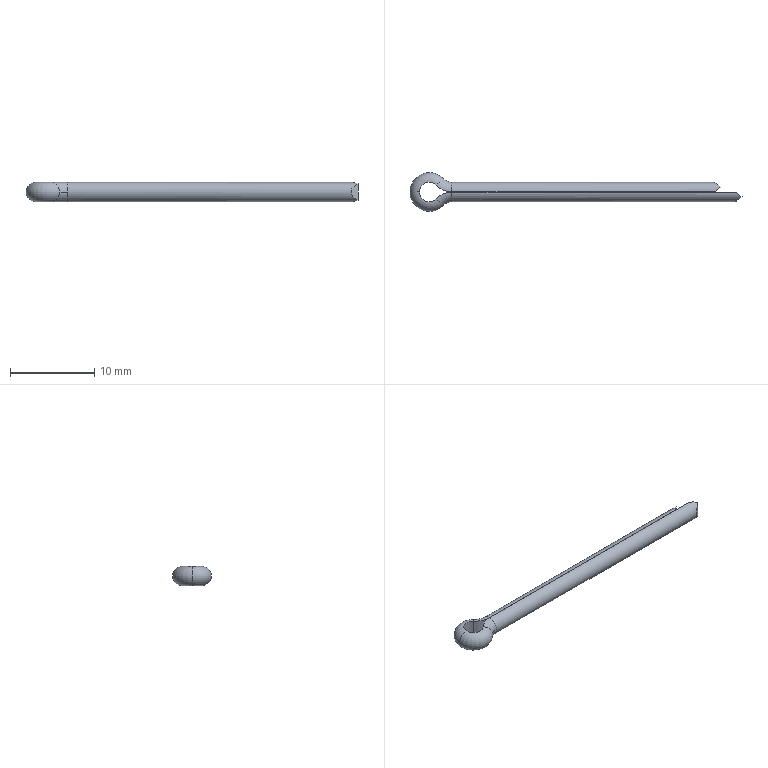Part | SolidWorks | features ICE 1, Sweep 1 | 1 solid | 17 faces | box 39.5 x 4.6 x 2.3 mm | volume 158.041 mm3 | torus 6 | plane 6 | cylinder 5 | commonest cylinder face diameters 2.3 x2 5.169 x2 2.32 x1
STEP:
#1=CARTESIAN_POINT('',(2.7,0.01,1.15));
#2=VERTEX_POINT('',#1);
#3=CARTESIAN_POINT('',(2.7,1.15,0.));
#4=VERTEX_POINT('',#3);
#5=CARTESIAN_POINT('',(2.7,0.,0.));
#6=DIRECTION('',(-1.,0.,0.));
#7=DIRECTION('',(0.,0.,1.));
#8=AXIS2_PLACEMENT_3D('',#5,#6,#7);
#9=CIRCLE('',#8,1.15);
#10=EDGE_CURVE('',#2,#4,#9,.T.);
#11=ORIENTED_EDGE('',*,*,#10,.T.);
#12=CARTESIAN_POINT('',(1.658,1.594,0.));
#13=VERTEX_POINT('',#12);
#14=CARTESIAN_POINT('',(2.7,2.595,0.));
#15=DIRECTION('',(0.,0.,-1.));
#16=DIRECTION('',(-1.,0.,0.));
#17=AXIS2_PLACEMENT_3D('',#14,#15,#16);
#18=CIRCLE('',#17,1.445);
#19=EDGE_CURVE('',#4,#13,#18,.T.);
#20=ORIENTED_EDGE('',*,*,#19,.T.);
#21=CARTESIAN_POINT('',(0.8364,0.8038,1.15));
#22=VERTEX_POINT('',#21);
#23=CARTESIAN_POINT('',(0.8292,0.7968,0.));
#24=DIRECTION('',(-0.6929,0.721,0.));
#25=DIRECTION('',(0.,0.,1.));
#26=AXIS2_PLACEMENT_3D('',#23,#24,#25);
#27=CIRCLE('',#26,1.15);
#28=EDGE_CURVE('',#22,#13,#27,.T.);
#29=ORIENTED_EDGE('',*,*,#28,.F.);
#30=CARTESIAN_POINT('',(2.7,2.595,1.15));
#31=DIRECTION('',(0.,0.,-1.));
#32=DIRECTION('',(-1.,0.,0.));
#33=AXIS2_PLACEMENT_3D('',#30,#31,#32);
#34=CIRCLE('',#33,2.585);
#35=EDGE_CURVE('',#2,#22,#34,.T.);
#36=ORIENTED_EDGE('',*,*,#35,.F.);
#37=EDGE_LOOP('',(#11,#20,#29,#36));
#38=FACE_OUTER_BOUND('',#37,.T.);
#39=CARTESIAN_POINT('',(2.7,2.595,0.));
#40=DIRECTION('',(0.,0.,-1.));
#41=DIRECTION('',(-1.,0.,0.));
#42=AXIS2_PLACEMENT_3D('',#39,#40,#41);
#43=TOROIDAL_SURFACE('',#42,2.595,1.15);
#44=ADVANCED_FACE('',(#38),#43,.T.);
#45=CARTESIAN_POINT('',(0.8364,-0.8038,1.15));
#46=VERTEX_POINT('',#45);
#47=CARTESIAN_POINT('',(1.658,-1.594,0.));
#48=VERTEX_POINT('',#47);
#49=CARTESIAN_POINT('',(0.8292,-0.7968,0.));
#50=DIRECTION('',(0.6929,0.721,0.));
#51=DIRECTION('',(0.,0.,1.));
#52=AXIS2_PLACEMENT_3D('',#49,#50,#51);
#53=CIRCLE('',#52,1.15);
#54=EDGE_CURVE('',#46,#48,#53,.T.);
#55=ORIENTED_EDGE('',*,*,#54,.T.);
#56=CARTESIAN_POINT('',(2.7,-1.15,0.));
#57=VERTEX_POINT('',#56);
#58=CARTESIAN_POINT('',(2.7,-2.595,0.));
#59=DIRECTION('',(0.,0.,-1.));
#60=DIRECTION('',(-1.,0.,0.));
#61=AXIS2_PLACEMENT_3D('',#58,#59,#60);
#62=CIRCLE('',#61,1.445);
#63=EDGE_CURVE('',#48,#57,#62,.T.);
#64=ORIENTED_EDGE('',*,*,#63,.T.);
#65=CARTESIAN_POINT('',(2.7,-0.01,1.15));
#66=VERTEX_POINT('',#65);
#67=CARTESIAN_POINT('',(2.7,0.,0.));
#68=DIRECTION('',(1.,0.,0.));
#69=DIRECTION('',(0.,0.,1.));
#70=AXIS2_PLACEMENT_3D('',#67,#68,#69);
#71=CIRCLE('',#70,1.15);
#72=EDGE_CURVE('',#66,#57,#71,.T.);
#73=ORIENTED_EDGE('',*,*,#72,.F.);
#74=CARTESIAN_POINT('',(2.7,-2.595,1.15));
#75=DIRECTION('',(0.,0.,-1.));
#76=DIRECTION('',(-1.,0.,0.));
#77=AXIS2_PLACEMENT_3D('',#74,#75,#76);
#78=CIRCLE('',#77,2.585);
#79=EDGE_CURVE('',#46,#66,#78,.T.);
#80=ORIENTED_EDGE('',*,*,#79,.F.);
#81=EDGE_LOOP('',(#55,#64,#73,#80));
#82=FACE_OUTER_BOUND('',#81,.T.);
#83=CARTESIAN_POINT('',(2.7,-2.595,0.));
#84=DIRECTION('',(0.,0.,-1.));
#85=DIRECTION('',(-1.,0.,0.));
#86=AXIS2_PLACEMENT_3D('',#83,#84,#85);
#87=TOROIDAL_SURFACE('',#86,2.595,1.15);
#88=ADVANCED_FACE('',(#82),#87,.T.);
#89=CARTESIAN_POINT('',(0.8364,0.8038,-1.15));
#90=VERTEX_POINT('',#89);
#91=CARTESIAN_POINT('',(-1.16,0.,-1.15));
#92=VERTEX_POINT('',#91);
#93=CARTESIAN_POINT('',(0.,0.,-1.15));
#94=DIRECTION('',(0.,0.,1.));
#95=DIRECTION('',(1.,0.,0.));
#96=AXIS2_PLACEMENT_3D('',#93,#94,#95);
#97=CIRCLE('',#96,1.16);
#98=EDGE_CURVE('',#90,#92,#97,.T.);
#99=ORIENTED_EDGE('',*,*,#98,.T.);
#100=CARTESIAN_POINT('',(-1.16,0.,1.15));
#101=VERTEX_POINT('',#100);
#102=CARTESIAN_POINT('',(-1.15,0.,0.));
#103=DIRECTION('',(0.,1.,0.));
#104=DIRECTION('',(-1.,0.,0.));
#105=AXIS2_PLACEMENT_3D('',#102,#103,#104);
#106=CIRCLE('',#105,1.15);
#107=EDGE_CURVE('',#92,#101,#106,.T.);
#108=ORIENTED_EDGE('',*,*,#107,.T.);
#109=CARTESIAN_POINT('',(0.,0.,1.15));
#110=DIRECTION('',(0.,0.,1.));
#111=DIRECTION('',(1.,0.,0.));
#112=AXIS2_PLACEMENT_3D('',#109,#110,#111);
#113=CIRCLE('',#112,1.16);
#114=EDGE_CURVE('',#22,#101,#113,.T.);
#115=ORIENTED_EDGE('',*,*,#114,.F.);
#116=ORIENTED_EDGE('',*,*,#28,.T.);
#117=CARTESIAN_POINT('',(0.8292,0.7968,0.));
#118=DIRECTION('',(-0.6929,0.721,0.));
#119=DIRECTION('',(0.,0.,1.));
#120=AXIS2_PLACEMENT_3D('',#117,#118,#119);
#121=CIRCLE('',#120,1.15);
#122=EDGE_CURVE('',#13,#90,#121,.T.);
#123=ORIENTED_EDGE('',*,*,#122,.T.);
#124=EDGE_LOOP('',(#99,#108,#115,#116,#123));
#125=FACE_OUTER_BOUND('',#124,.T.);
#126=CARTESIAN_POINT('',(0.,0.,0.));
#127=DIRECTION('',(0.,0.,1.));
#128=DIRECTION('',(1.,0.,0.));
#129=AXIS2_PLACEMENT_3D('',#126,#127,#128);
#130=TOROIDAL_SURFACE('',#129,1.15,1.15);
#131=ADVANCED_FACE('',(#125),#130,.T.);
#132=CARTESIAN_POINT('',(37.2,-0.58,-0.993));
#133=VERTEX_POINT('',#132);
#134=CARTESIAN_POINT('',(36.396,-0.01,-1.15));
#135=VERTEX_POINT('',#134);
#136=CARTESIAN_POINT('',(37.2,-0.58,-0.993));
#137=CARTESIAN_POINT('',(36.955,-0.4059,-1.095));
#138=CARTESIAN_POINT('',(36.681,-0.2116,-1.148));
#139=CARTESIAN_POINT('',(36.396,-0.01,-1.15));
#140=(BOUNDED_CURVE()B_SPLINE_CURVE(3,(#136,#137,#138,#139),.UNSPECIFIED.,.F.,.F.)B_SPLINE_CURVE_WITH_KNOTS((4,4),(1.042,1.562),.UNSPECIFIED.)CURVE()GEOMETRIC_REPRESENTATION_ITEM()RATIONAL_B_SPLINE_CURVE((1.,0.9776,0.9776,1.))REPRESENTATION_ITEM(''));
#141=EDGE_CURVE('',#133,#135,#140,.T.);
#142=ORIENTED_EDGE('',*,*,#141,.F.);
#143=CARTESIAN_POINT('',(37.2,-0.58,0.993));
#144=VERTEX_POINT('',#143);
#145=CARTESIAN_POINT('',(37.2,-0.58,0.993));
#146=CARTESIAN_POINT('',(35.965,-1.434,0.4944));
#147=CARTESIAN_POINT('',(35.965,-1.434,-0.4944));
#148=CARTESIAN_POINT('',(37.2,-0.58,-0.993));
#149=(BOUNDED_CURVE()B_SPLINE_CURVE(3,(#145,#146,#147,#148),.UNSPECIFIED.,.F.,.F.)B_SPLINE_CURVE_WITH_KNOTS((4,4),(2.099,4.184),.UNSPECIFIED.)CURVE()GEOMETRIC_REPRESENTATION_ITEM()RATIONAL_B_SPLINE_CURVE((1.,0.6696,0.6696,1.))REPRESENTATION_ITEM(''));
#150=EDGE_CURVE('',#144,#133,#149,.T.);
#151=ORIENTED_EDGE('',*,*,#150,.F.);
#152=CARTESIAN_POINT('',(36.396,-0.01,1.15));
#153=VERTEX_POINT('',#152);
#154=CARTESIAN_POINT('',(36.396,-0.01,1.15));
#155=CARTESIAN_POINT('',(36.681,-0.2116,1.148));
#156=CARTESIAN_POINT('',(36.955,-0.4059,1.095));
#157=CARTESIAN_POINT('',(37.2,-0.58,0.993));
#158=(BOUNDED_CURVE()B_SPLINE_CURVE(3,(#154,#155,#156,#157),.UNSPECIFIED.,.F.,.T.)B_SPLINE_CURVE_WITH_KNOTS((4,4),(4.721,5.241),.UNSPECIFIED.)CURVE()GEOMETRIC_REPRESENTATION_ITEM()RATIONAL_B_SPLINE_CURVE((1.,0.9776,0.9776,1.))REPRESENTATION_ITEM(''));
#159=EDGE_CURVE('',#153,#144,#158,.T.);
#160=ORIENTED_EDGE('',*,*,#159,.F.);
#161=CARTESIAN_POINT('',(2.7,-0.01,1.15));
#162=DIRECTION('',(1.,0.,0.));
#163=VECTOR('',#162,1000.);
#164=LINE('',#161,#163);
#165=EDGE_CURVE('',#66,#153,#164,.T.);
#166=ORIENTED_EDGE('',*,*,#165,.F.);
#167=ORIENTED_EDGE('',*,*,#72,.T.);
#168=CARTESIAN_POINT('',(2.7,-0.01,-1.15));
#169=VERTEX_POINT('',#168);
#170=CARTESIAN_POINT('',(2.7,0.,0.));
#171=DIRECTION('',(1.,0.,0.));
#172=DIRECTION('',(0.,0.,1.));
#173=AXIS2_PLACEMENT_3D('',#170,#171,#172);
#174=CIRCLE('',#173,1.15);
#175=EDGE_CURVE('',#57,#169,#174,.T.);
#176=ORIENTED_EDGE('',*,*,#175,.T.);
#177=CARTESIAN_POINT('',(2.7,-0.01,-1.15));
#178=DIRECTION('',(1.,0.,0.));
#179=VECTOR('',#178,1000.);
#180=LINE('',#177,#179);
#181=EDGE_CURVE('',#169,#135,#180,.T.);
#182=ORIENTED_EDGE('',*,*,#181,.T.);
#183=EDGE_LOOP('',(#142,#151,#160,#166,#167,#176,#182));
#184=FACE_OUTER_BOUND('',#183,.T.);
#185=CARTESIAN_POINT('',(2.7,0.,0.));
#186=DIRECTION('',(1.,0.,0.));
#187=DIRECTION('',(0.,1.,0.));
#188=AXIS2_PLACEMENT_3D('',#185,#186,#187);
#189=CYLINDRICAL_SURFACE('',#188,1.15);
#190=ADVANCED_FACE('',(#184),#189,.T.);
#191=CARTESIAN_POINT('',(36.396,-0.01,-1.15));
#192=DIRECTION('',(0.,0.,1.));
#193=VECTOR('',#192,1000.);
#194=LINE('',#191,#193);
#195=EDGE_CURVE('',#135,#153,#194,.T.);
#196=ORIENTED_EDGE('',*,*,#195,.F.);
#197=ORIENTED_EDGE('',*,*,#181,.F.);
#198=CARTESIAN_POINT('',(2.7,-0.01,-1.15));
#199=DIRECTION('',(0.,0.,1.));
#200=VECTOR('',#199,1000.);
#201=LINE('',#198,#200);
#202=EDGE_CURVE('',#169,#66,#201,.T.);
#203=ORIENTED_EDGE('',*,*,#202,.T.);
#204=ORIENTED_EDGE('',*,*,#165,.T.);
#205=EDGE_LOOP('',(#196,#197,#203,#204));
#206=FACE_OUTER_BOUND('',#205,.T.);
#207=CARTESIAN_POINT('',(2.7,-0.01,-1.15));
#208=DIRECTION('',(0.,1.,0.));
#209=DIRECTION('',(-1.,0.,0.));
#210=AXIS2_PLACEMENT_3D('',#207,#208,#209);
#211=PLANE('',#210);
#212=ADVANCED_FACE('',(#206),#211,.T.);
#213=CARTESIAN_POINT('',(0.8364,-0.8038,-1.15));
#214=VERTEX_POINT('',#213);
#215=CARTESIAN_POINT('',(0.8364,-0.8038,-1.15));
#216=DIRECTION('',(0.,0.,1.));
#217=VECTOR('',#216,1000.);
#218=LINE('',#215,#217);
#219=EDGE_CURVE('',#214,#46,#218,.T.);
#220=ORIENTED_EDGE('',*,*,#219,.T.);
#221=ORIENTED_EDGE('',*,*,#79,.T.);
#222=ORIENTED_EDGE('',*,*,#202,.F.);
#223=CARTESIAN_POINT('',(2.7,-2.595,-1.15));
#224=DIRECTION('',(0.,0.,-1.));
#225=DIRECTION('',(-1.,0.,0.));
#226=AXIS2_PLACEMENT_3D('',#223,#224,#225);
#227=CIRCLE('',#226,2.585);
#228=EDGE_CURVE('',#214,#169,#227,.T.);
#229=ORIENTED_EDGE('',*,*,#228,.F.);
#230=EDGE_LOOP('',(#220,#221,#222,#229));
#231=FACE_OUTER_BOUND('',#230,.T.);
#232=CARTESIAN_POINT('',(2.7,-2.595,0.));
#233=DIRECTION('',(0.,0.,-1.));
#234=DIRECTION('',(-1.,0.,0.));
#235=AXIS2_PLACEMENT_3D('',#232,#233,#234);
#236=CYLINDRICAL_SURFACE('',#235,2.585);
#237=ADVANCED_FACE('',(#231),#236,.T.);
#238=ORIENTED_EDGE('',*,*,#63,.F.);
#239=CARTESIAN_POINT('',(0.8292,-0.7968,0.));
#240=DIRECTION('',(0.6929,0.721,0.));
#241=DIRECTION('',(0.,0.,1.));
#242=AXIS2_PLACEMENT_3D('',#239,#240,#241);
#243=CIRCLE('',#242,1.15);
#244=EDGE_CURVE('',#48,#214,#243,.T.);
#245=ORIENTED_EDGE('',*,*,#244,.T.);
#246=ORIENTED_EDGE('',*,*,#228,.T.);
#247=ORIENTED_EDGE('',*,*,#175,.F.);
#248=EDGE_LOOP('',(#238,#245,#246,#247));
#249=FACE_OUTER_BOUND('',#248,.T.);
#250=CARTESIAN_POINT('',(2.7,-2.595,0.));
#251=DIRECTION('',(0.,0.,-1.));
#252=DIRECTION('',(-1.,0.,0.));
#253=AXIS2_PLACEMENT_3D('',#250,#251,#252);
#254=TOROIDAL_SURFACE('',#253,2.595,1.15);
#255=ADVANCED_FACE('',(#249),#254,.T.);
#256=CARTESIAN_POINT('',(0.8364,0.8038,-1.15));
#257=DIRECTION('',(0.,0.,1.));
#258=VECTOR('',#257,1000.);
#259=LINE('',#256,#258);
#260=EDGE_CURVE('',#90,#22,#259,.T.);
#261=ORIENTED_EDGE('',*,*,#260,.T.);
#262=ORIENTED_EDGE('',*,*,#114,.T.);
#263=CARTESIAN_POINT('',(0.,0.,1.15));
#264=DIRECTION('',(0.,0.,1.));
#265=DIRECTION('',(1.,0.,0.));
#266=AXIS2_PLACEMENT_3D('',#263,#264,#265);
#267=CIRCLE('',#266,1.16);
#268=EDGE_CURVE('',#101,#46,#267,.T.);
#269=ORIENTED_EDGE('',*,*,#268,.T.);
#270=ORIENTED_EDGE('',*,*,#219,.F.);
#271=CARTESIAN_POINT('',(0.,0.,-1.15));
#272=DIRECTION('',(0.,0.,1.));
#273=DIRECTION('',(1.,0.,0.));
#274=AXIS2_PLACEMENT_3D('',#271,#272,#273);
#275=CIRCLE('',#274,1.16);
#276=EDGE_CURVE('',#92,#214,#275,.T.);
#277=ORIENTED_EDGE('',*,*,#276,.F.);
#278=ORIENTED_EDGE('',*,*,#98,.F.);
#279=EDGE_LOOP('',(#261,#262,#269,#270,#277,#278));
#280=FACE_OUTER_BOUND('',#279,.T.);
#281=CARTESIAN_POINT('',(0.,0.,0.));
#282=DIRECTION('',(0.,0.,1.));
#283=DIRECTION('',(1.,0.,0.));
#284=AXIS2_PLACEMENT_3D('',#281,#282,#283);
#285=CYLINDRICAL_SURFACE('',#284,1.16);
#286=ADVANCED_FACE('',(#280),#285,.F.);
#287=ORIENTED_EDGE('',*,*,#107,.F.);
#288=ORIENTED_EDGE('',*,*,#276,.T.);
#289=ORIENTED_EDGE('',*,*,#244,.F.);
#290=ORIENTED_EDGE('',*,*,#54,.F.);
#291=ORIENTED_EDGE('',*,*,#268,.F.);
#292=EDGE_LOOP('',(#287,#288,#289,#290,#291));
#293=FACE_OUTER_BOUND('',#292,.T.);
#294=CARTESIAN_POINT('',(0.,0.,0.));
#295=DIRECTION('',(0.,0.,1.));
#296=DIRECTION('',(1.,0.,0.));
#297=AXIS2_PLACEMENT_3D('',#294,#295,#296);
#298=TOROIDAL_SURFACE('',#297,1.15,1.15);
#299=ADVANCED_FACE('',(#293),#298,.T.);
#300=CARTESIAN_POINT('',(2.7,0.01,-1.15));
#301=VERTEX_POINT('',#300);
#302=CARTESIAN_POINT('',(2.7,0.01,-1.15));
#303=DIRECTION('',(0.,0.,1.));
#304=VECTOR('',#303,1000.);
#305=LINE('',#302,#304);
#306=EDGE_CURVE('',#301,#2,#305,.T.);
#307=ORIENTED_EDGE('',*,*,#306,.T.);
#308=ORIENTED_EDGE('',*,*,#35,.T.);
#309=ORIENTED_EDGE('',*,*,#260,.F.);
#310=CARTESIAN_POINT('',(2.7,2.595,-1.15));
#311=DIRECTION('',(0.,0.,-1.));
#312=DIRECTION('',(-1.,0.,0.));
#313=AXIS2_PLACEMENT_3D('',#310,#311,#312);
#314=CIRCLE('',#313,2.585);
#315=EDGE_CURVE('',#301,#90,#314,.T.);
#316=ORIENTED_EDGE('',*,*,#315,.F.);
#317=EDGE_LOOP('',(#307,#308,#309,#316));
#318=FACE_OUTER_BOUND('',#317,.T.);
#319=CARTESIAN_POINT('',(2.7,2.595,0.));
#320=DIRECTION('',(0.,0.,-1.));
#321=DIRECTION('',(-1.,0.,0.));
#322=AXIS2_PLACEMENT_3D('',#319,#320,#321);
#323=CYLINDRICAL_SURFACE('',#322,2.585);
#324=ADVANCED_FACE('',(#318),#323,.T.);
#325=ORIENTED_EDGE('',*,*,#19,.F.);
#326=CARTESIAN_POINT('',(2.7,0.,0.));
#327=DIRECTION('',(-1.,0.,0.));
#328=DIRECTION('',(0.,0.,1.));
#329=AXIS2_PLACEMENT_3D('',#326,#327,#328);
#330=CIRCLE('',#329,1.15);
#331=EDGE_CURVE('',#4,#301,#330,.T.);
#332=ORIENTED_EDGE('',*,*,#331,.T.);
#333=ORIENTED_EDGE('',*,*,#315,.T.);
#334=ORIENTED_EDGE('',*,*,#122,.F.);
#335=EDGE_LOOP('',(#325,#332,#333,#334));
#336=FACE_OUTER_BOUND('',#335,.T.);
#337=CARTESIAN_POINT('',(2.7,2.595,0.));
#338=DIRECTION('',(0.,0.,-1.));
#339=DIRECTION('',(-1.,0.,0.));
#340=AXIS2_PLACEMENT_3D('',#337,#338,#339);
#341=TOROIDAL_SURFACE('',#340,2.595,1.15);
#342=ADVANCED_FACE('',(#336),#341,.T.);
#343=CARTESIAN_POINT('',(33.89,0.01,1.15));
#344=VERTEX_POINT('',#343);
#345=CARTESIAN_POINT('',(2.7,0.01,1.15));
#346=DIRECTION('',(1.,0.,0.));
#347=VECTOR('',#346,1000.);
#348=LINE('',#345,#347);
#349=EDGE_CURVE('',#2,#344,#348,.T.);
#350=ORIENTED_EDGE('',*,*,#349,.T.);
#351=CARTESIAN_POINT('',(34.7,0.57,0.9988));
#352=VERTEX_POINT('',#351);
#353=CARTESIAN_POINT('',(33.89,0.01,1.15));
#354=CARTESIAN_POINT('',(34.176,0.2076,1.148));
#355=CARTESIAN_POINT('',(34.452,0.3984,1.097));
#356=CARTESIAN_POINT('',(34.7,0.57,0.9988));
#357=(BOUNDED_CURVE()B_SPLINE_CURVE(3,(#353,#354,#355,#356),.UNSPECIFIED.,.F.,.F.)B_SPLINE_CURVE_WITH_KNOTS((4,4),(4.721,5.231),.UNSPECIFIED.)CURVE()GEOMETRIC_REPRESENTATION_ITEM()RATIONAL_B_SPLINE_CURVE((1.,0.9785,0.9785,1.))REPRESENTATION_ITEM(''));
#358=EDGE_CURVE('',#344,#352,#357,.T.);
#359=ORIENTED_EDGE('',*,*,#358,.T.);
#360=CARTESIAN_POINT('',(34.7,0.57,-0.9988));
#361=VERTEX_POINT('',#360);
#362=CARTESIAN_POINT('',(34.7,0.57,0.9988));
#363=CARTESIAN_POINT('',(33.472,1.441,0.5016));
#364=CARTESIAN_POINT('',(33.472,1.441,-0.5016));
#365=CARTESIAN_POINT('',(34.7,0.57,-0.9988));
#366=(BOUNDED_CURVE()B_SPLINE_CURVE(3,(#362,#363,#364,#365),.UNSPECIFIED.,.F.,.T.)B_SPLINE_CURVE_WITH_KNOTS((4,4),(2.089,4.194),.UNSPECIFIED.)CURVE()GEOMETRIC_REPRESENTATION_ITEM()RATIONAL_B_SPLINE_CURVE((1.,0.6638,0.6638,1.))REPRESENTATION_ITEM(''));
#367=EDGE_CURVE('',#352,#361,#366,.T.);
#368=ORIENTED_EDGE('',*,*,#367,.T.);
#369=CARTESIAN_POINT('',(33.89,0.01,-1.15));
#370=VERTEX_POINT('',#369);
#371=CARTESIAN_POINT('',(34.7,0.57,-0.9988));
#372=CARTESIAN_POINT('',(34.452,0.3984,-1.097));
#373=CARTESIAN_POINT('',(34.176,0.2076,-1.148));
#374=CARTESIAN_POINT('',(33.89,0.01,-1.15));
#375=(BOUNDED_CURVE()B_SPLINE_CURVE(3,(#371,#372,#373,#374),.UNSPECIFIED.,.F.,.F.)B_SPLINE_CURVE_WITH_KNOTS((4,4),(1.052,1.562),.UNSPECIFIED.)CURVE()GEOMETRIC_REPRESENTATION_ITEM()RATIONAL_B_SPLINE_CURVE((1.,0.9785,0.9785,1.))REPRESENTATION_ITEM(''));
#376=EDGE_CURVE('',#361,#370,#375,.T.);
#377=ORIENTED_EDGE('',*,*,#376,.T.);
#378=CARTESIAN_POINT('',(2.7,0.01,-1.15));
#379=DIRECTION('',(1.,0.,0.));
#380=VECTOR('',#379,1000.);
#381=LINE('',#378,#380);
#382=EDGE_CURVE('',#301,#370,#381,.T.);
#383=ORIENTED_EDGE('',*,*,#382,.F.);
#384=ORIENTED_EDGE('',*,*,#331,.F.);
#385=ORIENTED_EDGE('',*,*,#10,.F.);
#386=EDGE_LOOP('',(#350,#359,#368,#377,#383,#384,#385));
#387=FACE_OUTER_BOUND('',#386,.T.);
#388=CARTESIAN_POINT('',(2.7,0.,0.));
#389=DIRECTION('',(1.,0.,0.));
#390=DIRECTION('',(0.,0.,-1.));
#391=AXIS2_PLACEMENT_3D('',#388,#389,#390);
#392=CYLINDRICAL_SURFACE('',#391,1.15);
#393=ADVANCED_FACE('',(#387),#392,.T.);
#394=ORIENTED_EDGE('',*,*,#382,.T.);
#395=CARTESIAN_POINT('',(33.89,0.01,-1.15));
#396=DIRECTION('',(0.,0.,1.));
#397=VECTOR('',#396,1000.);
#398=LINE('',#395,#397);
#399=EDGE_CURVE('',#370,#344,#398,.T.);
#400=ORIENTED_EDGE('',*,*,#399,.T.);
#401=ORIENTED_EDGE('',*,*,#349,.F.);
#402=ORIENTED_EDGE('',*,*,#306,.F.);
#403=EDGE_LOOP('',(#394,#400,#401,#402));
#404=FACE_OUTER_BOUND('',#403,.T.);
#405=CARTESIAN_POINT('',(2.7,0.01,-1.15));
#406=DIRECTION('',(0.,1.,0.));
#407=DIRECTION('',(0.,0.,1.));
#408=AXIS2_PLACEMENT_3D('',#405,#406,#407);
#409=PLANE('',#408);
#410=ADVANCED_FACE('',(#404),#409,.F.);
#411=CARTESIAN_POINT('',(34.7,0.57,-1.15));
#412=DIRECTION('',(0.,0.,1.));
#413=VECTOR('',#412,1000.);
#414=LINE('',#411,#413);
#415=EDGE_CURVE('',#361,#352,#414,.T.);
#416=ORIENTED_EDGE('',*,*,#415,.T.);
#417=ORIENTED_EDGE('',*,*,#358,.F.);
#418=ORIENTED_EDGE('',*,*,#399,.F.);
#419=ORIENTED_EDGE('',*,*,#376,.F.);
#420=EDGE_LOOP('',(#416,#417,#418,#419));
#421=FACE_OUTER_BOUND('',#420,.T.);
#422=CARTESIAN_POINT('',(34.7,0.57,-1.15));
#423=DIRECTION('',(-0.5686,0.8226,0.));
#424=DIRECTION('',(-0.8226,-0.5686,0.));
#425=AXIS2_PLACEMENT_3D('',#422,#423,#424);
#426=PLANE('',#425);
#427=ADVANCED_FACE('',(#421),#426,.F.);
#428=ORIENTED_EDGE('',*,*,#415,.F.);
#429=ORIENTED_EDGE('',*,*,#367,.F.);
#430=EDGE_LOOP('',(#428,#429));
#431=FACE_OUTER_BOUND('',#430,.T.);
#432=CARTESIAN_POINT('',(34.7,0.57,-1.15));
#433=DIRECTION('',(-0.5786,-0.8156,0.));
#434=DIRECTION('',(0.8156,-0.5786,0.));
#435=AXIS2_PLACEMENT_3D('',#432,#433,#434);
#436=PLANE('',#435);
#437=ADVANCED_FACE('',(#431),#436,.F.);
#438=ORIENTED_EDGE('',*,*,#150,.T.);
#439=CARTESIAN_POINT('',(37.2,-0.58,-1.15));
#440=DIRECTION('',(0.,0.,1.));
#441=VECTOR('',#440,1000.);
#442=LINE('',#439,#441);
#443=EDGE_CURVE('',#133,#144,#442,.T.);
#444=ORIENTED_EDGE('',*,*,#443,.T.);
#445=EDGE_LOOP('',(#438,#444));
#446=FACE_OUTER_BOUND('',#445,.T.);
#447=CARTESIAN_POINT('',(37.2,-0.58,-1.15));
#448=DIRECTION('',(-0.5686,0.8226,0.));
#449=DIRECTION('',(-0.8226,-0.5686,0.));
#450=AXIS2_PLACEMENT_3D('',#447,#448,#449);
#451=PLANE('',#450);
#452=ADVANCED_FACE('',(#446),#451,.F.);
#453=ORIENTED_EDGE('',*,*,#141,.T.);
#454=ORIENTED_EDGE('',*,*,#195,.T.);
#455=ORIENTED_EDGE('',*,*,#159,.T.);
#456=ORIENTED_EDGE('',*,*,#443,.F.);
#457=EDGE_LOOP('',(#453,#454,#455,#456));
#458=FACE_OUTER_BOUND('',#457,.T.);
#459=CARTESIAN_POINT('',(37.2,-0.58,-1.15));
#460=DIRECTION('',(-0.5786,-0.8156,0.));
#461=DIRECTION('',(0.8156,-0.5786,0.));
#462=AXIS2_PLACEMENT_3D('',#459,#460,#461);
#463=PLANE('',#462);
#464=ADVANCED_FACE('',(#458),#463,.F.);
#465=CLOSED_SHELL('',(#44,#88,#131,#190,#212,#237,#255,#286,#299,#324,#342,#393,#410,#427,#437,#452,#464));
#466=MANIFOLD_SOLID_BREP('',#465);
#467=CARTESIAN_POINT('',(0.,0.,0.));
#468=DIRECTION('',(0.,0.,1.));
#469=DIRECTION('',(1.,0.,0.));
#470=AXIS2_PLACEMENT_3D('',#467,#468,#469);
#471=(LENGTH_UNIT()NAMED_UNIT(*)SI_UNIT(.MILLI.,.METRE.));
#472=UNCERTAINTY_MEASURE_WITH_UNIT(LENGTH_MEASURE(0.00001),#471,'','');
#473=(NAMED_UNIT(*)PLANE_ANGLE_UNIT()SI_UNIT($,.RADIAN.));
#474=(NAMED_UNIT(*)SI_UNIT($,.STERADIAN.)SOLID_ANGLE_UNIT());
#475=(GEOMETRIC_REPRESENTATION_CONTEXT(3)GLOBAL_UNCERTAINTY_ASSIGNED_CONTEXT((#472))GLOBAL_UNIT_ASSIGNED_CONTEXT((#471,#473,#474))REPRESENTATION_CONTEXT('',''));
#476=ADVANCED_BREP_SHAPE_REPRESENTATION('',(#466,#470),#475);